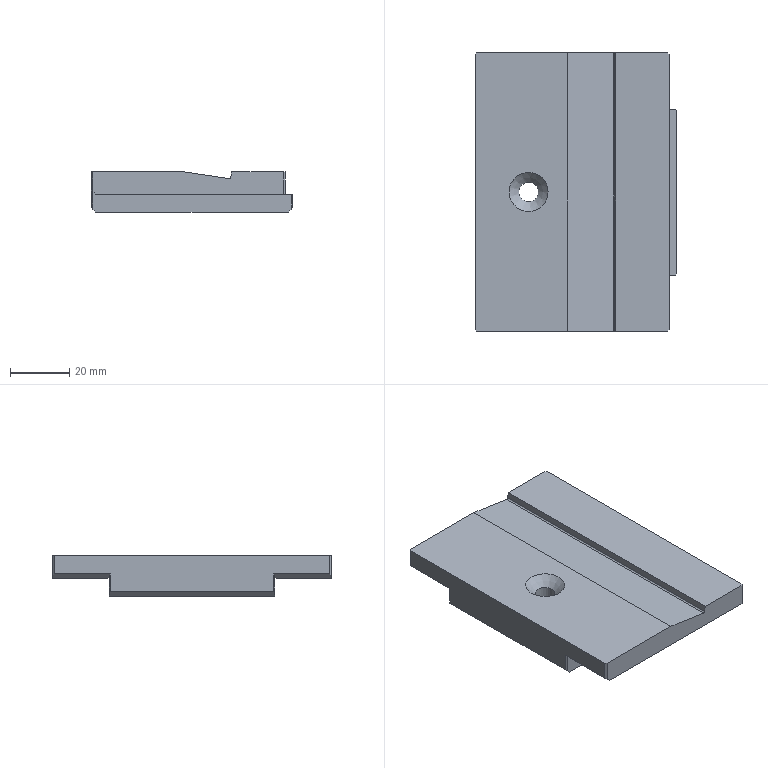NC program | NX | posted with a generic post | part box 68 x 94 x 13.65 mm
Lines 1098 to 1988 of 5620:
(CURVE_DRIVE , TOOL : D4R0.5)
N2152 T07 M6
N2154 G54
N2156 G17 G0 G90 X2.01 Y-11.204 B0. C0. S6500 M3
N2158 G43 Z30. H7
N2160 Z2.994
N2162 G94 G1 Z1.844 F1000.
N2164 X1.998 Y-11.205 Z1.635
N2166 X1.964 Z1.428
N2168 X1.909 Y-11.207 Z1.226
N2170 X1.833 Y-11.209 Z1.031
N2172 X1.737 Y-11.211 Z0.845
N2174 X1.622 Y-11.214 Z0.67
N2176 X1.489 Y-11.217 Z0.508
N2178 X1.341 Y-11.221 Z0.361
N2180 X1.177 Y-11.225 Z0.23
N2182 X1.001 Y-11.229 Z0.117
N2184 X0.814 Y-11.234 Z0.023
N2186 X0.618 Y-11.238 Z-0.051
N2188 X0.416 Y-11.243 Z-0.104
N2190 X0.209 Y-11.248 Z-0.136
N2192 X0. Y-11.254 Z-0.146
N2194 X-0.233 Y-11.259 Z-0.144
N2196 X-0.465 Y-11.276
N2198 X-0.696 Y-11.305
N2200 X-0.926 Y-11.345
N2202 X-1.153 Y-11.396 Z-0.145
N2204 X-1.378 Y-11.458
N2206 X-1.599 Y-11.531 Z-0.144
N2208 X-1.816 Y-11.615
N2210 X-2.029 Y-11.709
N2212 X-2.237 Y-11.814
N2214 X-2.44 Y-11.929 Z-0.145
N2216 X-2.637 Y-12.053
N2218 X-2.827 Y-12.188 Z-0.144
N2220 X-3.011 Y-12.331
N2222 X-3.188 Y-12.483
N2224 X-3.356 Y-12.644 Z-0.145
N2226 X-3.517 Y-12.812
N2228 X-3.669 Y-12.989 Z-0.144
N2230 X-3.812 Y-13.173
N2232 X-3.947 Y-13.363
N2234 X-4.071 Y-13.56
N2236 X-4.186 Y-13.763 Z-0.145
N2238 X-4.291 Y-13.971
N2240 X-4.385 Y-14.184 Z-0.144
N2242 X-4.469 Y-14.401
N2244 X-4.542 Y-14.622
N2246 X-4.604 Y-14.847 Z-0.145
N2248 X-4.655 Y-15.074
N2250 X-4.695 Y-15.304 Z-0.144
N2252 X-4.724 Y-15.535
N2254 X-4.741 Y-15.767
N2256 X-4.746 Y-16.
N2258 X-4.741 Y-16.233 Z-0.145
N2260 X-4.724 Y-16.465
N2262 X-4.695 Y-16.696 Z-0.144
N2264 X-4.655 Y-16.926
N2266 X-4.604 Y-17.153
N2268 X-4.542 Y-17.378
N2270 X-4.469 Y-17.599 Z-0.146
N2272 X-4.385 Y-17.816 Z-0.144
N2274 X-4.291 Y-18.029
N2276 X-4.186 Y-18.237
N2278 X-4.071 Y-18.44
N2280 X-3.947 Y-18.637 Z-0.145
N2282 X-3.812 Y-18.827
N2284 X-3.669 Y-19.011 Z-0.144
N2286 X-3.517 Y-19.188
N2288 X-3.356 Y-19.356
N2290 X-3.188 Y-19.517
N2292 X-3.011 Y-19.669 Z-0.145
N2294 X-2.827 Y-19.812 Z-0.144
N2296 X-2.637 Y-19.947
N2298 X-2.44 Y-20.071
N2300 X-2.237 Y-20.186
N2302 X-2.029 Y-20.291 Z-0.145
N2304 X-1.816 Y-20.385
N2306 X-1.599 Y-20.469 Z-0.144
N2308 X-1.378 Y-20.542
N2310 X-1.153 Y-20.604
N2312 X-0.926 Y-20.655
N2314 X-0.696 Y-20.695 Z-0.145
N2316 X-0.465 Y-20.724
N2318 X-0.233 Y-20.741 Z-0.144
N2320 X0. Y-20.746
N2322 X0.233 Y-20.741
N2324 X0.465 Y-20.724 Z-0.145
N2326 X0.696 Y-20.695
N2328 X0.926 Y-20.655 Z-0.144
N2330 X1.153 Y-20.604
N2332 X1.378 Y-20.542
N2334 X1.599 Y-20.469
N2336 X1.816 Y-20.385 Z-0.145
N2338 X2.029 Y-20.291
N2340 X2.237 Y-20.186 Z-0.144
N2342 X2.44 Y-20.071
N2344 X2.637 Y-19.947
N2346 X2.827 Y-19.812
N2348 X3.011 Y-19.669 Z-0.145
N2350 X3.188 Y-19.517 Z-0.144
N2352 X3.356 Y-19.356
N2354 X3.517 Y-19.188
N2356 X3.669 Y-19.011
N2358 X3.812 Y-18.827 Z-0.145
N2360 X3.947 Y-18.637
N2362 X4.071 Y-18.44 Z-0.144
N2364 X4.186 Y-18.237
N2366 X4.291 Y-18.029
N2368 X4.385 Y-17.816
N2370 X4.469 Y-17.599 Z-0.146
N2372 X4.542 Y-17.378 Z-0.144
N2374 X4.604 Y-17.153
N2376 X4.655 Y-16.926
N2378 X4.695 Y-16.696
N2380 X4.724 Y-16.465 Z-0.145
N2382 X4.741 Y-16.233
N2384 X4.746 Y-16. Z-0.144
N2386 X4.741 Y-15.767
N2388 X4.724 Y-15.535
N2390 X4.695 Y-15.304
N2392 X4.655 Y-15.074 Z-0.145
N2394 X4.604 Y-14.847
N2396 X4.542 Y-14.622 Z-0.144
N2398 X4.469 Y-14.401
N2400 X4.385 Y-14.184
N2402 X4.291 Y-13.971 Z-0.145
N2404 X4.186 Y-13.763
N2406 X4.071 Y-13.56 Z-0.144
N2408 X3.947 Y-13.363
N2410 X3.812 Y-13.173
N2412 X3.669 Y-12.989
N2414 X3.517 Y-12.812 Z-0.145
N2416 X3.356 Y-12.644
N2418 X3.188 Y-12.483 Z-0.144
N2420 X3.011 Y-12.331
N2422 X2.827 Y-12.188
N2424 X2.637 Y-12.053 Z-0.145
N2426 X2.44 Y-11.929
N2428 X2.237 Y-11.814 Z-0.144
N2430 X2.029 Y-11.709
N2432 X1.816 Y-11.615
N2434 X1.599 Y-11.531
N2436 X1.378 Y-11.458 Z-0.145
N2438 X1.153 Y-11.396
N2440 X0.926 Y-11.345 Z-0.144
N2442 X0.696 Y-11.305
N2444 X0.465 Y-11.276
N2446 X0.233 Y-11.259
N2448 X0. Y-11.254 Z-0.146
N2450 X-0.233 Y-11.26 Z-0.145
N2452 X-0.465 Y-11.278
N2454 X-0.696 Y-11.307 Z-0.146
N2456 X-0.925 Y-11.348 Z-0.147
N2458 X-1.152 Y-11.399 Z-0.149
N2460 X-1.377 Y-11.462
N2462 X-1.597 Y-11.536
N2464 X-1.814 Y-11.62
N2466 X-2.027 Y-11.715 Z-0.15
N2468 X-2.234 Y-11.821 Z-0.152
N2470 X-2.436 Y-11.936 Z-0.154
N2472 X-2.632 Y-12.061 Z-0.153
N2474 X-2.822 Y-12.195
N2476 X-3.005 Y-12.339 Z-0.154
N2478 X-3.18 Y-12.491 Z-0.155
N2480 X-3.348 Y-12.652 Z-0.156
N2482 X-3.508 Y-12.821 Z-0.158
N2484 X-3.659 Y-12.997 Z-0.157
N2486 X-3.801 Y-13.181 Z-0.158
N2488 X-3.934 Y-13.371
N2490 X-4.058 Y-13.568 Z-0.16
N2492 X-4.172 Y-13.77 Z-0.161
N2494 X-4.275 Y-13.978 Z-0.162
N2496 X-4.369 Y-14.19 Z-0.161
N2498 X-4.452 Y-14.407 Z-0.162
N2500 X-4.524 Y-14.628 Z-0.163
N2502 X-4.585 Y-14.852 Z-0.164
N2504 X-4.635 Y-15.078 Z-0.166
N2506 X-4.674 Y-15.307
N2508 X-4.702 Y-15.537
N2510 X-4.718 Y-15.768
N2512 X-4.723 Y-16. Z-0.168
N2514 X-4.716 Y-16.232 Z-0.169
N2516 X-4.699 Y-16.463 Z-0.17
N2518 X-4.67 Y-16.693
N2520 X-4.629 Y-16.921
N2522 X-4.578 Y-17.147 Z-0.171
N2524 X-4.515 Y-17.37 Z-0.172
N2526 X-4.442 Y-17.589 Z-0.174
N2528 X-4.358 Y-17.805
N2530 X-4.263 Y-18.016
N2532 X-4.159 Y-18.223
N2534 X-4.044 Y-18.424 Z-0.176
N2536 X-3.92 Y-18.619 Z-0.177
N2538 X-3.786 Y-18.808 Z-0.178
N2540 X-3.643 Y-18.99
N2542 X-3.491 Y-19.164
N2544 X-3.331 Y-19.331 Z-0.179
N2546 X-3.163 Y-19.49 Z-0.18
N2548 X-2.988 Y-19.641 Z-0.182
N2550 X-2.805 Y-19.782
N2552 X-2.616 Y-19.915
N2554 X-2.42 Y-20.038 Z-0.183
N2556 X-2.219 Y-20.151 Z-0.184
N2558 X-2.012 Y-20.254 Z-0.185
N2560 X-1.801 Y-20.347 Z-0.186
N2562 X-1.585 Y-20.429
N2564 X-1.365 Y-20.501
N2566 X-1.143 Y-20.562 Z-0.187
N2568 X-0.917 Y-20.612 Z-0.188
N2570 X-0.69 Y-20.651 Z-0.19
N2572 X-0.461 Y-20.678
N2574 X-0.231 Y-20.694
N2576 X0. Y-20.699 Z-0.191
N2578 X0.231 Y-20.693 Z-0.192
N2580 X0.46 Y-20.675 Z-0.193
N2582 X0.689 Y-20.646 Z-0.195
N2584 X0.916 Y-20.606 Z-0.194
N2586 X1.141 Y-20.555
N2588 X1.363 Y-20.493 Z-0.195
N2590 X1.581 Y-20.42 Z-0.196
N2592 X1.796 Y-20.336 Z-0.198
N2594 X2.006 Y-20.242 Z-0.199
N2596 X2.212 Y-20.138 Z-0.198
N2598 X2.412 Y-20.024 Z-0.199
N2600 X2.606 Y-19.9 Z-0.2
N2602 X2.794 Y-19.767 Z-0.201
N2604 X2.975 Y-19.625 Z-0.203
N2606 X3.148 Y-19.474 Z-0.202
N2608 X3.315 Y-19.315 Z-0.203
N2610 X3.473 Y-19.147
N2612 X3.622 Y-18.973 Z-0.204
N2614 X3.763 Y-18.791 Z-0.206
N2616 X3.895 Y-18.603 Z-0.207
N2618 X4.017 Y-18.408
N2620 X4.13 Y-18.208
N2622 X4.233 Y-18.002 Z-0.208
N2624 X4.325 Y-17.792 Z-0.209
N2626 X4.407 Y-17.577 Z-0.211
N2628 X4.479 Y-17.359
N2630 X4.539 Y-17.137
N2632 X4.589 Y-16.913
N2634 X4.627 Y-16.686 Z-0.212
N2636 X4.655 Y-16.458 Z-0.214
N2638 X4.671 Y-16.229 Z-0.215
N2640 X4.676 Y-16.
N2642 X4.669 Y-15.771
N2644 X4.652 Y-15.542 Z-0.216
N2646 X4.623 Y-15.314 Z-0.217
N2648 X4.583 Y-15.088 Z-0.219
N2650 X4.532 Y-14.865
N2652 X4.47 Y-14.644
N2654 X4.398 Y-14.427
N2656 X4.314 Y-14.213 Z-0.22
N2658 X4.221 Y-14.004 Z-0.222
N2660 X4.117 Y-13.799 Z-0.223
N2662 X4.004 Y-13.6
N2664 X3.88 Y-13.407
N2666 X3.748 Y-13.22 Z-0.224
N2668 X3.606 Y-13.04 Z-0.225
N2670 X3.456 Y-12.867 Z-0.227
N2672 X3.298 Y-12.702
N2674 X3.132 Y-12.545
N2676 X2.958 Y-12.396 Z-0.228
N2678 X2.777 Y-12.256
N2680 X2.59 Y-12.125 Z-0.23
N2682 X2.396 Y-12.003 Z-0.232
N2684 X2.196 Y-11.891 Z-0.231
N2686 X1.992 Y-11.789
N2688 X1.783 Y-11.697 Z-0.232
N2690 X1.569 Y-11.615 Z-0.233
N2692 X1.352 Y-11.544 Z-0.235
N2694 X1.131 Y-11.484
N2696 X0.908 Y-11.434
N2698 X0.683 Y-11.396 Z-0.236
N2700 X0.456 Y-11.369 Z-0.237
N2702 X0.228 Y-11.353 Z-0.238
N2704 X0. Y-11.348 Z-0.24
N2706 X-0.228 Y-11.354 Z-0.239
N2708 X-0.456 Y-11.372
N2710 X-0.682 Y-11.4 Z-0.24
N2712 X-0.907 Y-11.44 Z-0.241
N2714 X-1.129 Y-11.491 Z-0.243
N2716 X-1.349 Y-11.552 Z-0.244
N2718 X-1.566 Y-11.625
N2720 X-1.778 Y-11.707
N2722 X-1.986 Y-11.8 Z-0.245
N2724 X-2.19 Y-11.904 Z-0.246
N2726 X-2.388 Y-12.017 Z-0.248
N2728 X-2.58 Y-12.139
N2730 X-2.766 Y-12.271
N2732 X-2.945 Y-12.412
N2734 X-3.117 Y-12.561 Z-0.249
N2736 X-3.281 Y-12.719 Z-0.251
N2738 X-3.438 Y-12.884 Z-0.252
N2740 X-3.586 Y-13.057
N2742 X-3.725 Y-13.237
N2744 X-3.856 Y-13.424 Z-0.253
N2746 X-3.977 Y-13.616 Z-0.254
N2748 X-4.089 Y-13.815 Z-0.256
N2750 X-4.19 Y-14.018
N2752 X-4.282 Y-14.226
N2754 X-4.363 Y-14.439
N2756 X-4.434 Y-14.655 Z-0.257
N2758 X-4.493 Y-14.874 Z-0.259
N2760 X-4.543 Y-15.096 Z-0.26
N2762 X-4.581 Y-15.321
N2764 X-4.608 Y-15.546
N2766 X-4.624 Y-15.773 Z-0.261
N2768 X-4.629 Y-16. Z-0.262
N2770 X-4.622 Y-16.227 Z-0.264
N2772 X-4.605 Y-16.454
N2774 X-4.576 Y-16.679
N2776 X-4.537 Y-16.902
N2778 X-4.486 Y-17.124 Z-0.265
N2780 X-4.425 Y-17.342 Z-0.267
N2782 X-4.353 Y-17.558 Z-0.269
N2784 X-4.271 Y-17.769 Z-0.268
N2786 X-4.178 Y-17.976
N2788 X-4.076 Y-18.178 Z-0.269
N2790 X-3.963 Y-18.375 Z-0.27
N2792 X-3.841 Y-18.567 Z-0.272
N2794 X-3.71 Y-18.752
N2796 X-3.57 Y-18.93
N2798 X-3.421 Y-19.101 Z-0.273
N2800 X-3.265 Y-19.265
N2802 X-3.1 Y-19.42 Z-0.275
N2804 X-2.928 Y-19.568 Z-0.277
N2806 X-2.749 Y-19.706 Z-0.276
N2808 X-2.563 Y-19.836
N2810 X-2.372 Y-19.957 Z-0.277
N2812 X-2.174 Y-20.068 Z-0.278
N2814 X-1.972 Y-20.169 Z-0.28
N2816 X-1.765 Y-20.26 Z-0.281
N2818 X-1.553 Y-20.341 Z-0.28
N2820 X-1.338 Y-20.411 Z-0.281
N2822 X-1.12 Y-20.471
N2824 X-0.899 Y-20.519 Z-0.283
N2826 X-0.676 Y-20.557 Z-0.285
N2828 X-0.452 Y-20.584
N2830 X-0.226 Y-20.6
N2832 X0. Y-20.605
N2834 X0.226 Y-20.599 Z-0.286
N2836 X0.451 Y-20.581 Z-0.288
N2838 X0.675 Y-20.553 Z-0.289
N2840 X0.898 Y-20.514
N2842 X1.118 Y-20.463
N2844 X1.335 Y-20.402
N2846 X1.55 Y-20.331 Z-0.291
N2848 X1.76 Y-20.249 Z-0.293
N2850 X1.966 Y-20.157
N2852 X2.167 Y-20.055
N2854 X2.363 Y-19.943
N2856 X2.554 Y-19.822 Z-0.294
N2858 X2.738 Y-19.691 Z-0.296
N2860 X2.915 Y-19.552 Z-0.297
N2862 X3.085 Y-19.404
N2864 X3.248 Y-19.248
N2866 X3.403 Y-19.084 Z-0.298
N2868 X3.549 Y-18.913 Z-0.299
N2870 X3.688 Y-18.735 Z-0.3
N2872 X3.817 Y-18.55 Z-0.301
N2874 X3.937 Y-18.36
N2876 X4.047 Y-18.163
N2878 X4.148 Y-17.962 Z-0.302
N2880 X4.238 Y-17.755 Z-0.304
N2882 X4.318 Y-17.545 Z-0.305
N2884 X4.388 Y-17.331
N2886 X4.448 Y-17.114
N2888 X4.496 Y-16.894 Z-0.306
N2890 X4.534 Y-16.673 Z-0.307
N2892 X4.561 Y-16.449 Z-0.308
N2894 X4.577 Y-16.225 Z-0.309
N2896 X4.581 Y-16.
N2898 X4.575 Y-15.775
N2900 X4.558 Y-15.551 Z-0.31
N2902 X4.53 Y-15.328 Z-0.311
N2904 X4.491 Y-15.107 Z-0.313
N2906 X4.441 Y-14.888
N2908 X4.38 Y-14.671
N2910 X4.309 Y-14.458 Z-0.314
N2912 X4.227 Y-14.249 Z-0.315
N2914 X4.136 Y-14.044 Z-0.316
N2916 X4.034 Y-13.844 Z-0.318
N2918 X3.923 Y-13.649 Z-0.317
N2920 X3.802 Y-13.46
N2922 X3.672 Y-13.277 Z-0.318
N2924 X3.534 Y-13.1 Z-0.32
N2926 X3.386 Y-12.931 Z-0.321
N2928 X3.231 Y-12.769 Z-0.322
N2930 X3.068 Y-12.615 Z-0.321
N2932 X2.898 Y-12.469 Z-0.322
N2934 X2.721 Y-12.331 Z-0.323
N2936 X2.537 Y-12.203 Z-0.324
N2938 X2.347 Y-12.084 Z-0.326
N2940 X2.152 Y-11.974
N2942 X1.952 Y-11.874
N2944 X1.746 Y-11.784
N2946 X1.537 Y-11.704 Z-0.328
N2948 X1.324 Y-11.634 Z-0.329
N2950 X1.108 Y-11.575 Z-0.33
N2952 X0.89 Y-11.527
N2954 X0.669 Y-11.489
N2956 X0.447 Y-11.463 Z-0.331
N2958 X0.224 Y-11.447 Z-0.332
N2960 X0. Y-11.442 Z-0.334
N2962 X-0.224 Y-11.448
N2964 X-0.447 Y-11.466
N2966 X-0.668 Y-11.494
N2968 X-0.889 Y-11.533 Z-0.335
N2970 X-1.107 Y-11.582 Z-0.337
N2972 X-1.322 Y-11.643 Z-0.338
N2974 X-1.534 Y-11.713
N2976 X-1.742 Y-11.795
N2978 X-1.946 Y-11.886 Z-0.339
N2980 X-2.145 Y-11.987 Z-0.34
N2982 X-2.339 Y-12.098 Z-0.342
N2984 X-2.527 Y-12.218
N2986 X-2.709 Y-12.347
N2988 X-2.885 Y-12.485 Z-0.343
N2990 X-3.053 Y-12.631 Z-0.344
N2992 X-3.215 Y-12.785 Z-0.345
N2994 X-3.368 Y-12.948 Z-0.346
N2996 X-3.513 Y-13.117
N2998 X-3.65 Y-13.293
N3000 X-3.777 Y-13.476 Z-0.347
N3002 X-3.896 Y-13.665 Z-0.348
N3004 X-4.005 Y-13.859 Z-0.35
N3006 X-4.105 Y-14.059
N3008 X-4.195 Y-14.263
N3010 X-4.274 Y-14.471 Z-0.351
N3012 X-4.343 Y-14.682 Z-0.352
N3014 X-4.402 Y-14.897 Z-0.353
N3016 X-4.45 Y-15.115 Z-0.355
N3018 X-4.487 Y-15.334 Z-0.354
N3020 X-4.514 Y-15.555
N3022 X-4.53 Y-15.777 Z-0.355
N3024 X-4.534 Y-16. Z-0.356
N3026 X-4.528 Y-16.222 Z-0.358
N3028 X-4.511 Y-16.444
N3030 X-4.483 Y-16.665
N3032 X-4.444 Y-16.884 Z-0.359
N3034 X-4.395 Y-17.101 Z-0.36
N3036 X-4.335 Y-17.315 Z-0.361
N3038 X-4.264 Y-17.526 Z-0.363
N3040 X-4.184 Y-17.733
N3042 X-4.093 Y-17.936
N3044 X-3.992 Y-18.134
N3046 X-3.882 Y-18.327 Z-0.364
N3048 X-3.763 Y-18.514 Z-0.366
N3050 X-3.634 Y-18.695 Z-0.367
N3052 X-3.497 Y-18.87 Z-0.366
N3054 X-3.352 Y-19.038 Z-0.367
N3056 X-3.198 Y-19.198 Z-0.368
N3058 X-3.037 Y-19.35 Z-0.369
N3060 X-2.868 Y-19.495 Z-0.371
N3062 X-2.693 Y-19.631
N3064 X-2.511 Y-19.758
N3066 X-2.323 Y-19.876
N3068 X-2.13 Y-19.985 Z-0.372
N3070 X-1.931 Y-20.084 Z-0.374
N3072 X-1.728 Y-20.173 Z-0.375
N3074 X-1.521 Y-20.252
N3076 X-1.311 Y-20.321
N3078 X-1.097 Y-20.379 Z-0.376
N3080 X-0.881 Y-20.427 Z-0.377
N3082 X-0.662 Y-20.464 Z-0.379
N3084 X-0.442 Y-20.49
N3086 X-0.221 Y-20.506
N3088 X0. Y-20.511
N3090 X0.221 Y-20.505 Z-0.38
N3092 X0.442 Y-20.488 Z-0.382
N3094 X0.662 Y-20.46 Z-0.383
N3096 X0.879 Y-20.421
N3098 X1.095 Y-20.372
N3100 X1.308 Y-20.312 Z-0.384
N3102 X1.518 Y-20.242 Z-0.385
N3104 X1.724 Y-20.162 Z-0.387
N3106 X1.926 Y-20.072
N3108 X2.123 Y-19.972
N3110 X2.315 Y-19.862
N3112 X2.501 Y-19.743 Z-0.388
N3114 X2.681 Y-19.615 Z-0.39
N3116 X2.855 Y-19.479 Z-0.392
N3118 X3.022 Y-19.334 Z-0.391
N3120 X3.181 Y-19.181
N3122 X3.333 Y-19.021 Z-0.392
N3124 X3.477 Y-18.853 Z-0.393
N3126 X3.612 Y-18.679 Z-0.395
N3128 X3.738 Y-18.498
N3130 X3.856 Y-18.311
N3132 X3.964 Y-18.119 Z-0.396
N3134 X4.062 Y-17.921
N3136 X4.151 Y-17.719 Z-0.398
N3138 X4.23 Y-17.513 Z-0.4
N3140 X4.298 Y-17.304 Z-0.399
N3142 X4.356 Y-17.091
N3144 X4.404 Y-16.876 Z-0.4
N3146 X4.441 Y-16.659 Z-0.401
N3148 X4.467 Y-16.44 Z-0.403
N3150 X4.482 Y-16.22 Z-0.404
N3152 X4.487 Y-16. Z-0.403
N3154 X4.481 Y-15.78 Z-0.404
N3156 X4.464 Y-15.56 Z-0.405
N3158 X4.436 Y-15.342 Z-0.406
N3160 X4.398 Y-15.125 Z-0.408
N3162 X4.349 Y-14.911
N3164 X4.29 Y-14.699
N3166 X4.22 Y-14.49
N3168 X4.14 Y-14.285 Z-0.409
N3170 X4.05 Y-14.084 Z-0.411
N3172 X3.951 Y-13.888 Z-0.412
N3174 X3.842 Y-13.697
N3176 X3.724 Y-13.512
N3178 X3.596 Y-13.333 Z-0.413
N3180 X3.461 Y-13.16 Z-0.414
N3182 X3.317 Y-12.994 Z-0.416
N3184 X3.165 Y-12.835
N3186 X3.005 Y-12.685
N3188 X2.838 Y-12.542
N3190 X2.665 Y-12.407 Z-0.417
N3192 X2.485 Y-12.281 Z-0.419
N3194 X2.299 Y-12.165 Z-0.42
N3196 X2.108 Y-12.057
N3198 X1.911 Y-11.959
N3200 X1.71 Y-11.871 Z-0.421
N3202 X1.505 Y-11.792 Z-0.422
N3204 X1.297 Y-11.724 Z-0.424
N3206 X1.085 Y-11.667
N3208 X0.871 Y-11.619
N3210 X0.655 Y-11.583
N3212 X0.438 Y-11.556 Z-0.425
N3214 X0.219 Y-11.541 Z-0.427
N3216 X0. Y-11.536 Z-0.428
N3218 X-0.219 Y-11.543
N3220 X-0.437 Y-11.559
N3222 X-0.655 Y-11.587 Z-0.429
N3224 X-0.87 Y-11.625 Z-0.43
N3226 X-1.084 Y-11.674 Z-0.432
N3228 X-1.294 Y-11.733
N3230 X-1.502 Y-11.802
N3232 X-1.706 Y-11.882
N3234 X-1.906 Y-11.971 Z-0.433
N3236 X-2.101 Y-12.07 Z-0.435
N3238 X-2.291 Y-12.178 Z-0.436
N3240 X-2.475 Y-12.296
N3242 X-2.653 Y-12.423
N3244 X-2.825 Y-12.558 Z-0.437
N3246 X-2.99 Y-12.701 Z-0.438
N3248 X-3.148 Y-12.852 Z-0.439
N3250 X-3.298 Y-13.011 Z-0.441
N3252 X-3.44 Y-13.177 Z-0.44
N3254 X-3.574 Y-13.349 Z-0.441
N3256 X-3.699 Y-13.528
N3258 X-3.815 Y-13.713 Z-0.443
N3260 X-3.922 Y-13.904 Z-0.444
N3262 X-4.02 Y-14.099 Z-0.445
N3264 X-4.107 Y-14.299
N3266 X-4.185 Y-14.502
N3268 X-4.253 Y-14.71 Z-0.446
N3270 X-4.311 Y-14.92 Z-0.447
N3272 X-4.358 Y-15.133 Z-0.449
N3274 X-4.394 Y-15.348
N3276 X-4.42 Y-15.565
N3278 X-4.435 Y-15.782
N3280 X-4.44 Y-16. Z-0.451
N3282 X-4.434 Y-16.218 Z-0.452
N3284 X-4.417 Y-16.435 Z-0.453
N3286 X-4.39 Y-16.651
N3288 X-4.352 Y-16.866
N3290 X-4.303 Y-17.078 Z-0.454
N3292 X-4.245 Y-17.288 Z-0.455
N3294 X-4.176 Y-17.494 Z-0.457
N3296 X-4.097 Y-17.697
N3298 X-4.008 Y-17.896
N3300 X-3.909 Y-18.09
N3302 X-3.801 Y-18.278 Z-0.459
N3304 X-3.684 Y-18.462 Z-0.46
N3306 X-3.559 Y-18.639 Z-0.461
N3308 X-3.424 Y-18.81
N3310 X-3.282 Y-18.974
N3312 X-3.131 Y-19.131 Z-0.462
N3314 X-2.973 Y-19.281 Z-0.463
N3316 X-2.808 Y-19.422 Z-0.465
N3318 X-2.637 Y-19.555
N3320 X-2.459 Y-19.679
N3322 X-2.275 Y-19.795 Z-0.466
N3324 X-2.085 Y-19.901 Z-0.467
N3326 X-1.891 Y-19.998 Z-0.468
N3328 X-1.692 Y-20.086 Z-0.469
N3330 X-1.49 Y-20.163
N3332 X-1.283 Y-20.231
N3334 X-1.074 Y-20.288 Z-0.47
N3336 X-0.862 Y-20.334 Z-0.471
N3338 X-0.648 Y-20.371 Z-0.473
N3340 X-0.433 Y-20.397
N3342 X-0.217 Y-20.412
N3344 X0. Y-20.416 Z-0.474
N3346 X0.217 Y-20.41 Z-0.475
N3348 X0.433 Y-20.394 Z-0.476
N3350 X0.648 Y-20.366 Z-0.478
N3352 X0.861 Y-20.329 Z-0.477
N3354 X1.072 Y-20.281 Z-0.478
N3356 X1.281 Y-20.222
N3358 X1.486 Y-20.153 Z-0.479
N3360 X1.688 Y-20.075 Z-0.481
N3362 X1.885 Y-19.986 Z-0.482
N3364 X2.078 Y-19.888 Z-0.481
N3366 X2.266 Y-19.781 Z-0.482
N3368 X2.449 Y-19.665 Z-0.483
N3370 X2.625 Y-19.54 Z-0.484
N3372 X2.795 Y-19.406 Z-0.486
N3374 X2.958 Y-19.264 Z-0.485
N3376 X3.115 Y-19.115 Z-0.486
N3378 X3.263 Y-18.957
N3380 X3.404 Y-18.793 Z-0.487
N3382 X3.536 Y-18.623 Z-0.489
N3384 X3.66 Y-18.445 Z-0.49
N3386 X3.775 Y-18.263
N3388 X3.881 Y-18.074
N3390 X3.977 Y-17.881 Z-0.491
N3392 X4.064 Y-17.683 Z-0.492
N3394 X4.141 Y-17.482 Z-0.494
N3396 X4.208 Y-17.276
N3398 X4.265 Y-17.068
N3400 X4.311 Y-16.858
N3402 X4.348 Y-16.645 Z-0.496
N3404 X4.373 Y-16.431 Z-0.497
N3406 X4.388 Y-16.216 Z-0.498
N3408 X4.393 Y-16.
N3410 X4.387 Y-15.784
N3412 X4.37 Y-15.57 Z-0.499
N3414 X4.343 Y-15.356 Z-0.5
N3416 X4.306 Y-15.144 Z-0.502
N3418 X4.258 Y-14.934
N3420 X4.199 Y-14.726
N3422 X4.131 Y-14.522
N3424 X4.053 Y-14.321 Z-0.503
N3426 X3.965 Y-14.125 Z-0.505
N3428 X3.868 Y-13.933 Z-0.506
N3430 X3.761 Y-13.746
N3432 X3.645 Y-13.564
N3434 X3.521 Y-13.389 Z-0.507
N3436 X3.388 Y-13.22 Z-0.508
N3438 X3.247 Y-13.057 Z-0.51
N3440 X3.098 Y-12.902
N3442 X2.942 Y-12.754
N3444 X2.778 Y-12.615 Z-0.511
N3446 X2.608 Y-12.483
N3448 X2.432 Y-12.36 Z-0.513
N3450 X2.25 Y-12.245 Z-0.515
N3452 X2.063 Y-12.14 Z-0.514
N3454 X1.871 Y-12.044
N3456 X1.674 Y-11.958 Z-0.515
N3458 X1.474 Y-11.881 Z-0.516
N3460 X1.27 Y-11.815 Z-0.518
N3462 X1.063 Y-11.758
N3464 X0.853 Y-11.712
N3466 X0.641 Y-11.676 Z-0.519
N3468 X0.428 Y-11.65 Z-0.52
N3470 X0.214 Y-11.635 Z-0.521
N3472 X0. Y-11.631 Z-0.523
N3474 X-0.214 Y-11.637 Z-0.522
N3476 X-0.428 Y-11.653 Z-0.523
N3478 X-0.641 Y-11.68
N3480 X-0.852 Y-11.718 Z-0.524
N3482 X-1.061 Y-11.765 Z-0.526
N3484 X-1.267 Y-11.823 Z-0.527
N3486 X-1.47 Y-11.891
N3488 X-1.67 Y-11.969
N3490 X-1.865 Y-12.056 Z-0.528
N3492 X-2.056 Y-12.153 Z-0.529
N3494 X-2.242 Y-12.259 Z-0.531
N3496 X-2.423 Y-12.374
N3498 X-2.597 Y-12.498
N3500 X-2.765 Y-12.63
N3502 X-2.927 Y-12.771 Z-0.532
N3504 X-3.081 Y-12.919 Z-0.534
N3506 X-3.228 Y-13.074 Z-0.535
N3508 X-3.367 Y-13.237
N3510 X-3.498 Y-13.406
N3512 X-3.621 Y-13.581 Z-0.536
N3514 X-3.734 Y-13.762 Z-0.537
N3516 X-3.839 Y-13.948 Z-0.539
N3518 X-3.934 Y-14.139
N3520 X-4.02 Y-14.335
N3522 X-4.097 Y-14.534
N3524 X-4.163 Y-14.737 Z-0.54
N3526 X-4.219 Y-14.943 Z-0.542
N3528 X-4.265 Y-15.152 Z-0.543
N3530 X-4.301 Y-15.362
N3532 X-4.326 Y-15.574
N3534 X-4.341 Y-15.787 Z-0.544
N3536 X-4.346 Y-16. Z-0.545
N3538 X-4.34 Y-16.213 Z-0.547
N3540 X-4.323 Y-16.426
N3542 X-4.297 Y-16.637
N3544 X-4.259 Y-16.847
N3546 X-4.212 Y-17.055 Z-0.548
N3548 X-4.154 Y-17.26 Z-0.55
N3550 X-4.087 Y-17.462 Z-0.552
N3552 X-4.009 Y-17.661 Z-0.551
N3554 X-3.923 Y-17.855
N3556 X-3.826 Y-18.045 Z-0.552
N3558 X-3.721 Y-18.23 Z-0.553
N3560 X-3.606 Y-18.409 Z-0.555
N3562 X-3.483 Y-18.583
N3564 X-3.351 Y-18.75
N3566 X-3.212 Y-18.911 Z-0.556
N3568 X-3.065 Y-19.065
N3570 X-2.91 Y-19.211 Z-0.558
N3572 X-2.748 Y-19.349 Z-0.56
N3574 X-2.58 Y-19.479 Z-0.559
N3576 X-2.406 Y-19.601
N3578 X-2.226 Y-19.714 Z-0.56
N3580 X-2.041 Y-19.818 Z-0.561
N3582 X-1.851 Y-19.913 Z-0.563
N3584 X-1.656 Y-19.999 Z-0.564
N3586 X-1.458 Y-20.074 Z-0.563
N3588 X-1.256 Y-20.14 Z-0.564
N3590 X-1.051 Y-20.196 Z-0.565
N3592 X-0.844 Y-20.242 Z-0.566
N3594 X-0.635 Y-20.278 Z-0.567
N3596 X-0.424 Y-20.303
N3598 X-0.212 Y-20.318 Z-0.568
N3600 X0. Y-20.322
N3602 X0.212 Y-20.316 Z-0.569
N3604 X0.424 Y-20.3 Z-0.57
N3606 X0.634 Y-20.273 Z-0.572
N3608 X0.843 Y-20.236
N3610 X1.049 Y-20.189
N3612 X1.253 Y-20.132
N3614 X1.454 Y-20.065 Z-0.574
N3616 X1.652 Y-19.988 Z-0.576
N3618 X1.845 Y-19.901
N3620 X2.034 Y-19.805
N3622 X2.218 Y-19.7
N3624 X2.396 Y-19.586 Z-0.577
N3626 X2.569 Y-19.464 Z-0.579
N3628 X2.735 Y-19.333 Z-0.58
N3630 X2.895 Y-19.194
N3632 X3.048 Y-19.048
N3634 X3.193 Y-18.894 Z-0.581
N3636 X3.331 Y-18.734 Z-0.582
N3638 X3.46 Y-18.566 Z-0.583
N3640 X3.581 Y-18.393 Z-0.584
N3642 X3.694 Y-18.214
N3644 X3.798 Y-18.03
N3646 X3.892 Y-17.841 Z-0.585
N3648 X3.977 Y-17.647 Z-0.587
N3650 X4.052 Y-17.45 Z-0.588
N3652 X4.118 Y-17.249
N3654 X4.173 Y-17.045
N3656 X4.219 Y-16.839 Z-0.589
N3658 X4.254 Y-16.631 Z-0.59
N3660 X4.279 Y-16.421 Z-0.591
N3662 X4.294 Y-16.211 Z-0.592
N3664 X4.299 Y-16.
N3666 X4.293 Y-15.789 Z-0.593
N3668 X4.276 Y-15.579
N3670 X4.25 Y-15.37 Z-0.594
N3672 X4.213 Y-15.162 Z-0.596
N3674 X4.166 Y-14.956
N3676 X4.109 Y-14.753
N3678 X4.042 Y-14.554 Z-0.597
N3680 X3.966 Y-14.357 Z-0.598
N3682 X3.88 Y-14.165 Z-0.599
N3684 X3.785 Y-13.977 Z-0.601
N3686 X3.68 Y-13.794 Z-0.6
N3688 X3.567 Y-13.617
N3690 X3.445 Y-13.445 Z-0.601
N3692 X3.315 Y-13.28 Z-0.603
N3694 X3.177 Y-13.121 Z-0.604
N3696 X3.031 Y-12.969
N3698 X2.878 Y-12.824 Z-0.605
N3700 X2.719 Y-12.687
N3702 X2.552 Y-12.559 Z-0.606
N3704 X2.38 Y-12.438 Z-0.607
N3706 X2.202 Y-12.326 Z-0.609
N3708 X2.019 Y-12.223
N3710 X1.831 Y-12.129
N3712 X1.638 Y-12.045
N3714 X1.442 Y-11.97 Z-0.611
N3716 X1.242 Y-11.905 Z-0.612
N3718 X1.04 Y-11.85 Z-0.613
N3720 X0.835 Y-11.804
N3722 X0.628 Y-11.769
N3724 X0.419 Y-11.744 Z-0.614
N3726 X0.21 Y-11.729 Z-0.615
N3728 X0. Y-11.725 Z-0.617
N3730 X-0.21 Y-11.731
N3732 X-0.419 Y-11.747
N3734 X-0.627 Y-11.773
N3736 X-0.833 Y-11.81 Z-0.618
N3738 X-1.038 Y-11.857 Z-0.62
N3740 X-1.24 Y-11.913 Z-0.621
N3742 X-1.438 Y-11.98
N3744 X-1.634 Y-12.056
N3746 X-1.825 Y-12.141 Z-0.622
N3748 X-2.012 Y-12.236 Z-0.623
N3750 X-2.194 Y-12.34 Z-0.625
N3752 X-2.37 Y-12.453
N3754 X-2.541 Y-12.574
N3756 X-2.706 Y-12.703 Z-0.626
N3758 X-2.864 Y-12.841 Z-0.627
N3760 X-3.015 Y-12.985 Z-0.628
N3762 X-3.158 Y-13.137 Z-0.629
N3764 X-3.294 Y-13.296
N3766 X-3.422 Y-13.462
N3768 X-3.542 Y-13.633 Z-0.63
N3770 X-3.654 Y-13.81 Z-0.631
N3772 X-3.756 Y-13.992 Z-0.633
N3774 X-3.849 Y-14.179
N3776 X-3.933 Y-14.371
N3778 X-4.008 Y-14.566 Z-0.634
N3780 X-4.073 Y-14.765 Z-0.635
N3782 X-4.128 Y-14.966 Z-0.636
N3784 X-4.173 Y-15.17 Z-0.638
N3786 X-4.208 Y-15.376 Z-0.637
N3788 X-4.232 Y-15.583
N3790 X-4.247 Y-15.791 Z-0.638
N3792 X-4.251 Y-16. Z-0.639
N3794 X-4.246 Y-16.209 Z-0.641
N3796 X-4.23 Y-16.417
N3798 X-4.203 Y-16.623
N3800 X-4.167 Y-16.829 Z-0.642
N3802 X-4.12 Y-17.032 Z-0.643
N3804 X-4.064 Y-17.233 Z-0.644
N3806 X-3.998 Y-17.431 Z-0.646
N3808 X-3.922 Y-17.625
N3810 X-3.837 Y-17.815 Z-0.645
N3812 X-3.743 Y-18.001 Z-0.646
N3814 X-3.64 Y-18.182 Z-0.647
N3816 X-3.528 Y-18.357 Z-0.649
N3818 X-3.407 Y-18.527 Z-0.65
N3820 X-3.278 Y-18.691 Z-0.649
N3822 X-3.142 Y-18.848 Z-0.65
N3824 X-2.998 Y-18.998 Z-0.651
N3826 X-2.847 Y-19.141 Z-0.652
N3828 X-2.689 Y-19.276 Z-0.654
N3830 X-2.524 Y-19.404
N3832 X-2.354 Y-19.523
N3834 X-2.178 Y-19.633
N3836 X-1.996 Y-19.735 Z-0.655
N3838 X-1.81 Y-19.828 Z-0.657
N3840 X-1.62 Y-19.911 Z-0.658
N3842 X-1.426 Y-19.986
N3844 X-1.229 Y-20.05
N3846 X-1.028 Y-20.105 Z-0.659
N3848 X-0.825 Y-20.15 Z-0.66
N3850 X-0.621 Y-20.184 Z-0.662
N3852 X-0.415 Y-20.209
N3854 X-0.207 Y-20.224
N3856 X0. Y-20.228 Z-0.663
N3858 X0.207 Y-20.222
N3860 X0.414 Y-20.206 Z-0.665
N3862 X0.62 Y-20.18 Z-0.666
N3864 X0.824 Y-20.144
N3866 X1.026 Y-20.098
N3868 X1.226 Y-20.042 Z-0.667
N3870 X1.423 Y-19.976 Z-0.668
N3872 X1.616 Y-19.901 Z-0.67
N3874 X1.805 Y-19.816
N3876 X1.99 Y-19.722
N3878 X2.169 Y-19.619
N3880 X2.344 Y-19.508 Z-0.672
N3882 X2.513 Y-19.388 Z-0.673
N3884 X2.676 Y-19.26 Z-0.675
N3886 X2.832 Y-19.124 Z-0.674
N3888 X2.981 Y-18.981
N3890 X3.123 Y-18.831 Z-0.675
N3892 X3.258 Y-18.674 Z-0.676
N3894 X3.385 Y-18.51 Z-0.678
N3896 X3.503 Y-18.341
N3898 X3.613 Y-18.166
N3900 X3.714 Y-17.985 Z-0.679
N3902 X3.807 Y-17.8
N3904 X3.89 Y-17.611 Z-0.681
N3906 X3.963 Y-17.418 Z-0.683
N3908 X4.027 Y-17.222 Z-0.682
N3910 X4.082 Y-17.022
N3912 X4.126 Y-16.821 Z-0.683
N3914 X4.161 Y-16.617 Z-0.684
N3916 X4.186 Y-16.412 Z-0.686
N3918 X4.2 Y-16.206 Z-0.687
N3920 X4.204 Y-16. Z-0.686
N3922 X4.199 Y-15.794 Z-0.687
N3924 X4.183 Y-15.588 Z-0.688
N3926 X4.157 Y-15.383 Z-0.689